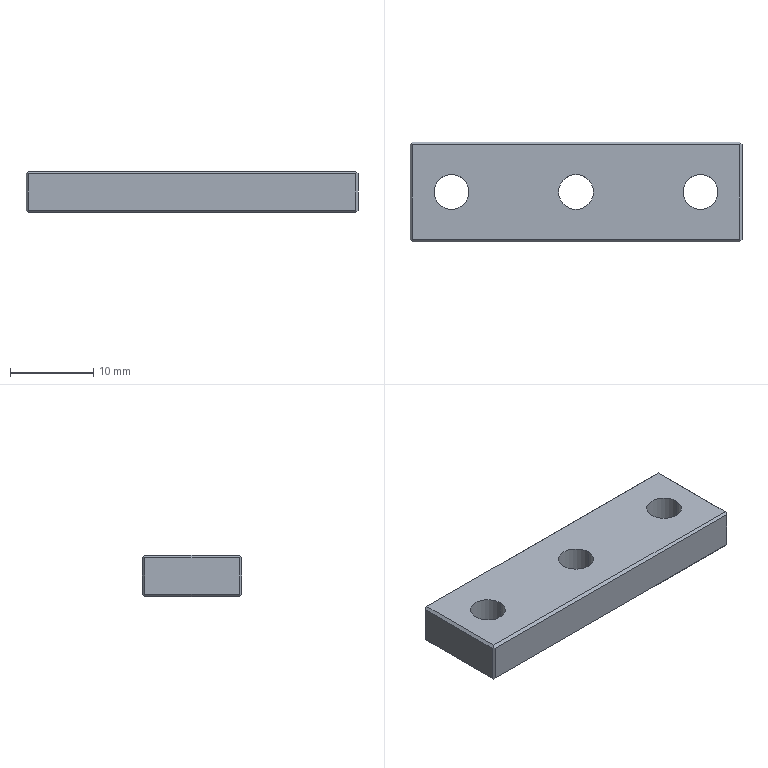Part | NX | 1 solid | 30 faces | box 40 x 12 x 5 mm | volume 2175 mm3 | plane 18 | cylinder 6 | cone 6 | commonest cylinder face diameters 4.2 x6
STEP:
#1=CARTESIAN_POINT('',(536.,16.4,-148.98));
#2=VERTEX_POINT('',#1);
#3=CARTESIAN_POINT('',(536.,16.4,-144.58));
#4=VERTEX_POINT('',#3);
#5=CARTESIAN_POINT('',(536.,16.4,-146.78));
#6=DIRECTION('',(0.,0.,1.));
#7=VECTOR('',#6,1000.);
#8=LINE('',#5,#7);
#9=EDGE_CURVE('',#2,#4,#8,.T.);
#10=ORIENTED_EDGE('',*,*,#9,.T.);
#11=CARTESIAN_POINT('',(536.,27.8,-144.58));
#12=VERTEX_POINT('',#11);
#13=CARTESIAN_POINT('',(536.,22.1,-144.58));
#14=DIRECTION('',(0.,1.,0.));
#15=VECTOR('',#14,1000.);
#16=LINE('',#13,#15);
#17=EDGE_CURVE('',#4,#12,#16,.T.);
#18=ORIENTED_EDGE('',*,*,#17,.T.);
#19=CARTESIAN_POINT('',(536.,27.8,-148.98));
#20=VERTEX_POINT('',#19);
#21=CARTESIAN_POINT('',(536.,27.8,-146.78));
#22=DIRECTION('',(0.,0.,1.));
#23=VECTOR('',#22,1000.);
#24=LINE('',#21,#23);
#25=EDGE_CURVE('',#20,#12,#24,.T.);
#26=ORIENTED_EDGE('',*,*,#25,.F.);
#27=CARTESIAN_POINT('',(536.,22.1,-148.98));
#28=DIRECTION('',(0.,1.,0.));
#29=VECTOR('',#28,1000.);
#30=LINE('',#27,#29);
#31=EDGE_CURVE('',#2,#20,#30,.T.);
#32=ORIENTED_EDGE('',*,*,#31,.F.);
#33=EDGE_LOOP('',(#10,#18,#26,#32));
#34=FACE_BOUND('',#33,.T.);
#35=CARTESIAN_POINT('',(536.,28.1,-144.28));
#36=DIRECTION('',(-1.,0.,0.));
#37=DIRECTION('',(0.,0.,1.));
#38=AXIS2_PLACEMENT_3D('',#35,#36,#37);
#39=PLANE('',#38);
#40=ADVANCED_FACE('',(#34),#39,.T.);
#41=CARTESIAN_POINT('',(575.7,28.1,-144.58));
#42=VERTEX_POINT('',#41);
#43=CARTESIAN_POINT('',(575.7,28.1,-148.98));
#44=VERTEX_POINT('',#43);
#45=CARTESIAN_POINT('',(575.7,28.1,-146.78));
#46=DIRECTION('',(0.,0.,-1.));
#47=VECTOR('',#46,1000.);
#48=LINE('',#45,#47);
#49=EDGE_CURVE('',#42,#44,#48,.T.);
#50=ORIENTED_EDGE('',*,*,#49,.T.);
#51=CARTESIAN_POINT('',(536.3,28.1,-148.98));
#52=VERTEX_POINT('',#51);
#53=CARTESIAN_POINT('',(556.,28.1,-148.98));
#54=DIRECTION('',(-1.,0.,0.));
#55=VECTOR('',#54,1000.);
#56=LINE('',#53,#55);
#57=EDGE_CURVE('',#44,#52,#56,.T.);
#58=ORIENTED_EDGE('',*,*,#57,.T.);
#59=CARTESIAN_POINT('',(536.3,28.1,-144.58));
#60=VERTEX_POINT('',#59);
#61=CARTESIAN_POINT('',(536.3,28.1,-146.78));
#62=DIRECTION('',(0.,0.,1.));
#63=VECTOR('',#62,1000.);
#64=LINE('',#61,#63);
#65=EDGE_CURVE('',#52,#60,#64,.T.);
#66=ORIENTED_EDGE('',*,*,#65,.T.);
#67=CARTESIAN_POINT('',(556.,28.1,-144.58));
#68=DIRECTION('',(-1.,0.,0.));
#69=VECTOR('',#68,1000.);
#70=LINE('',#67,#69);
#71=EDGE_CURVE('',#42,#60,#70,.T.);
#72=ORIENTED_EDGE('',*,*,#71,.F.);
#73=EDGE_LOOP('',(#50,#58,#66,#72));
#74=FACE_BOUND('',#73,.T.);
#75=CARTESIAN_POINT('',(596.,28.1,-144.28));
#76=DIRECTION('',(0.,1.,0.));
#77=DIRECTION('',(1.,0.,0.));
#78=AXIS2_PLACEMENT_3D('',#75,#76,#77);
#79=PLANE('',#78);
#80=ADVANCED_FACE('',(#74),#79,.T.);
#81=CARTESIAN_POINT('',(576.,16.4,-144.58));
#82=VERTEX_POINT('',#81);
#83=CARTESIAN_POINT('',(576.,16.4,-148.98));
#84=VERTEX_POINT('',#83);
#85=CARTESIAN_POINT('',(576.,16.4,-146.78));
#86=DIRECTION('',(0.,0.,-1.));
#87=VECTOR('',#86,1000.);
#88=LINE('',#85,#87);
#89=EDGE_CURVE('',#82,#84,#88,.T.);
#90=ORIENTED_EDGE('',*,*,#89,.T.);
#91=CARTESIAN_POINT('',(576.,27.8,-148.98));
#92=VERTEX_POINT('',#91);
#93=CARTESIAN_POINT('',(576.,22.1,-148.98));
#94=DIRECTION('',(0.,-1.,0.));
#95=VECTOR('',#94,1000.);
#96=LINE('',#93,#95);
#97=EDGE_CURVE('',#92,#84,#96,.T.);
#98=ORIENTED_EDGE('',*,*,#97,.F.);
#99=CARTESIAN_POINT('',(576.,27.8,-144.58));
#100=VERTEX_POINT('',#99);
#101=CARTESIAN_POINT('',(576.,27.8,-146.78));
#102=DIRECTION('',(0.,0.,-1.));
#103=VECTOR('',#102,1000.);
#104=LINE('',#101,#103);
#105=EDGE_CURVE('',#100,#92,#104,.T.);
#106=ORIENTED_EDGE('',*,*,#105,.F.);
#107=CARTESIAN_POINT('',(576.,22.1,-144.58));
#108=DIRECTION('',(0.,-1.,0.));
#109=VECTOR('',#108,1000.);
#110=LINE('',#107,#109);
#111=EDGE_CURVE('',#100,#82,#110,.T.);
#112=ORIENTED_EDGE('',*,*,#111,.T.);
#113=EDGE_LOOP('',(#90,#98,#106,#112));
#114=FACE_BOUND('',#113,.T.);
#115=CARTESIAN_POINT('',(576.,17.1,-144.28));
#116=DIRECTION('',(1.,0.,0.));
#117=DIRECTION('',(0.,1.,0.));
#118=AXIS2_PLACEMENT_3D('',#115,#116,#117);
#119=PLANE('',#118);
#120=ADVANCED_FACE('',(#114),#119,.T.);
#121=CARTESIAN_POINT('',(575.7,16.1,-144.58));
#122=VERTEX_POINT('',#121);
#123=CARTESIAN_POINT('',(536.3,16.1,-144.58));
#124=VERTEX_POINT('',#123);
#125=CARTESIAN_POINT('',(556.,16.1,-144.58));
#126=DIRECTION('',(-1.,0.,0.));
#127=VECTOR('',#126,1000.);
#128=LINE('',#125,#127);
#129=EDGE_CURVE('',#122,#124,#128,.T.);
#130=ORIENTED_EDGE('',*,*,#129,.T.);
#131=CARTESIAN_POINT('',(536.3,16.1,-148.98));
#132=VERTEX_POINT('',#131);
#133=CARTESIAN_POINT('',(536.3,16.1,-146.78));
#134=DIRECTION('',(0.,0.,1.));
#135=VECTOR('',#134,1000.);
#136=LINE('',#133,#135);
#137=EDGE_CURVE('',#132,#124,#136,.T.);
#138=ORIENTED_EDGE('',*,*,#137,.F.);
#139=CARTESIAN_POINT('',(575.7,16.1,-148.98));
#140=VERTEX_POINT('',#139);
#141=CARTESIAN_POINT('',(556.,16.1,-148.98));
#142=DIRECTION('',(-1.,0.,0.));
#143=VECTOR('',#142,1000.);
#144=LINE('',#141,#143);
#145=EDGE_CURVE('',#140,#132,#144,.T.);
#146=ORIENTED_EDGE('',*,*,#145,.F.);
#147=CARTESIAN_POINT('',(575.7,16.1,-146.78));
#148=DIRECTION('',(0.,0.,-1.));
#149=VECTOR('',#148,1000.);
#150=LINE('',#147,#149);
#151=EDGE_CURVE('',#122,#140,#150,.T.);
#152=ORIENTED_EDGE('',*,*,#151,.F.);
#153=EDGE_LOOP('',(#130,#138,#146,#152));
#154=FACE_BOUND('',#153,.T.);
#155=CARTESIAN_POINT('',(516.,16.1,-144.28));
#156=DIRECTION('',(0.,-1.,0.));
#157=DIRECTION('',(0.,0.,-1.));
#158=AXIS2_PLACEMENT_3D('',#155,#156,#157);
#159=PLANE('',#158);
#160=ADVANCED_FACE('',(#154),#159,.T.);
#161=ORIENTED_EDGE('',*,*,#89,.F.);
#162=CARTESIAN_POINT('',(575.85,16.25,-144.43));
#163=VERTEX_POINT('',#162);
#164=CARTESIAN_POINT('',(555.747,-3.853,-124.327));
#165=DIRECTION('',(-0.5774,-0.5774,0.5774));
#166=VECTOR('',#165,1000.);
#167=LINE('',#164,#166);
#168=EDGE_CURVE('',#82,#163,#167,.T.);
#169=ORIENTED_EDGE('',*,*,#168,.T.);
#170=CARTESIAN_POINT('',(555.747,-3.853,-164.533));
#171=DIRECTION('',(-0.5774,-0.5774,-0.5774));
#172=VECTOR('',#171,1000.);
#173=LINE('',#170,#172);
#174=EDGE_CURVE('',#163,#122,#173,.T.);
#175=ORIENTED_EDGE('',*,*,#174,.T.);
#176=ORIENTED_EDGE('',*,*,#151,.T.);
#177=CARTESIAN_POINT('',(575.85,16.25,-149.13));
#178=VERTEX_POINT('',#177);
#179=CARTESIAN_POINT('',(555.747,-3.853,-129.027));
#180=DIRECTION('',(-0.5774,-0.5774,0.5774));
#181=VECTOR('',#180,1000.);
#182=LINE('',#179,#181);
#183=EDGE_CURVE('',#178,#140,#182,.T.);
#184=ORIENTED_EDGE('',*,*,#183,.F.);
#185=CARTESIAN_POINT('',(555.747,-3.853,-169.233));
#186=DIRECTION('',(-0.5774,-0.5774,-0.5774));
#187=VECTOR('',#186,1000.);
#188=LINE('',#185,#187);
#189=EDGE_CURVE('',#84,#178,#188,.T.);
#190=ORIENTED_EDGE('',*,*,#189,.F.);
#191=EDGE_LOOP('',(#161,#169,#175,#176,#184,#190));
#192=FACE_BOUND('',#191,.T.);
#193=CARTESIAN_POINT('',(575.85,16.25,-146.78));
#194=DIRECTION('',(0.7071,-0.7071,0.));
#195=DIRECTION('',(0.,0.,-1.));
#196=AXIS2_PLACEMENT_3D('',#193,#194,#195);
#197=PLANE('',#196);
#198=ADVANCED_FACE('',(#192),#197,.T.);
#199=ORIENTED_EDGE('',*,*,#49,.F.);
#200=CARTESIAN_POINT('',(575.85,27.95,-144.43));
#201=VERTEX_POINT('',#200);
#202=CARTESIAN_POINT('',(607.653,-3.853,-112.627));
#203=DIRECTION('',(-0.5774,0.5774,-0.5774));
#204=VECTOR('',#203,1000.);
#205=LINE('',#202,#204);
#206=EDGE_CURVE('',#201,#42,#205,.T.);
#207=ORIENTED_EDGE('',*,*,#206,.F.);
#208=CARTESIAN_POINT('',(607.653,-3.853,-176.233));
#209=DIRECTION('',(0.5774,-0.5774,-0.5774));
#210=VECTOR('',#209,1000.);
#211=LINE('',#208,#210);
#212=EDGE_CURVE('',#201,#100,#211,.T.);
#213=ORIENTED_EDGE('',*,*,#212,.T.);
#214=ORIENTED_EDGE('',*,*,#105,.T.);
#215=CARTESIAN_POINT('',(575.85,27.95,-149.13));
#216=VERTEX_POINT('',#215);
#217=CARTESIAN_POINT('',(607.653,-3.853,-117.327));
#218=DIRECTION('',(0.5774,-0.5774,0.5774));
#219=VECTOR('',#218,1000.);
#220=LINE('',#217,#219);
#221=EDGE_CURVE('',#216,#92,#220,.T.);
#222=ORIENTED_EDGE('',*,*,#221,.F.);
#223=CARTESIAN_POINT('',(607.653,-3.853,-180.933));
#224=DIRECTION('',(-0.5774,0.5774,0.5774));
#225=VECTOR('',#224,1000.);
#226=LINE('',#223,#225);
#227=EDGE_CURVE('',#216,#44,#226,.T.);
#228=ORIENTED_EDGE('',*,*,#227,.T.);
#229=EDGE_LOOP('',(#199,#207,#213,#214,#222,#228));
#230=FACE_BOUND('',#229,.T.);
#231=CARTESIAN_POINT('',(575.85,27.95,-146.78));
#232=DIRECTION('',(0.7071,0.7071,0.));
#233=DIRECTION('',(0.,0.,-1.));
#234=AXIS2_PLACEMENT_3D('',#231,#232,#233);
#235=PLANE('',#234);
#236=ADVANCED_FACE('',(#230),#235,.T.);
#237=ORIENTED_EDGE('',*,*,#25,.T.);
#238=CARTESIAN_POINT('',(536.15,27.95,-144.43));
#239=VERTEX_POINT('',#238);
#240=CARTESIAN_POINT('',(504.347,-3.853,-176.233));
#241=DIRECTION('',(-0.5774,-0.5774,-0.5774));
#242=VECTOR('',#241,1000.);
#243=LINE('',#240,#242);
#244=EDGE_CURVE('',#239,#12,#243,.T.);
#245=ORIENTED_EDGE('',*,*,#244,.F.);
#246=CARTESIAN_POINT('',(504.347,-3.853,-112.627));
#247=DIRECTION('',(0.5774,0.5774,-0.5774));
#248=VECTOR('',#247,1000.);
#249=LINE('',#246,#248);
#250=EDGE_CURVE('',#239,#60,#249,.T.);
#251=ORIENTED_EDGE('',*,*,#250,.T.);
#252=ORIENTED_EDGE('',*,*,#65,.F.);
#253=CARTESIAN_POINT('',(536.15,27.95,-149.13));
#254=VERTEX_POINT('',#253);
#255=CARTESIAN_POINT('',(504.347,-3.853,-180.933));
#256=DIRECTION('',(0.5774,0.5774,0.5774));
#257=VECTOR('',#256,1000.);
#258=LINE('',#255,#257);
#259=EDGE_CURVE('',#254,#52,#258,.T.);
#260=ORIENTED_EDGE('',*,*,#259,.F.);
#261=CARTESIAN_POINT('',(504.347,-3.853,-117.327));
#262=DIRECTION('',(-0.5774,-0.5774,0.5774));
#263=VECTOR('',#262,1000.);
#264=LINE('',#261,#263);
#265=EDGE_CURVE('',#254,#20,#264,.T.);
#266=ORIENTED_EDGE('',*,*,#265,.T.);
#267=EDGE_LOOP('',(#237,#245,#251,#252,#260,#266));
#268=FACE_BOUND('',#267,.T.);
#269=CARTESIAN_POINT('',(536.15,27.95,-146.78));
#270=DIRECTION('',(0.7071,-0.7071,0.));
#271=DIRECTION('',(0.,0.,-1.));
#272=AXIS2_PLACEMENT_3D('',#269,#270,#271);
#273=PLANE('',#272);
#274=ADVANCED_FACE('',(#268),#273,.F.);
#275=ORIENTED_EDGE('',*,*,#9,.F.);
#276=CARTESIAN_POINT('',(536.15,16.25,-149.13));
#277=VERTEX_POINT('',#276);
#278=CARTESIAN_POINT('',(556.253,-3.853,-169.233));
#279=DIRECTION('',(-0.5774,0.5774,0.5774));
#280=VECTOR('',#279,1000.);
#281=LINE('',#278,#280);
#282=EDGE_CURVE('',#277,#2,#281,.T.);
#283=ORIENTED_EDGE('',*,*,#282,.F.);
#284=CARTESIAN_POINT('',(556.253,-3.853,-129.027));
#285=DIRECTION('',(-0.5774,0.5774,-0.5774));
#286=VECTOR('',#285,1000.);
#287=LINE('',#284,#286);
#288=EDGE_CURVE('',#132,#277,#287,.T.);
#289=ORIENTED_EDGE('',*,*,#288,.F.);
#290=ORIENTED_EDGE('',*,*,#137,.T.);
#291=CARTESIAN_POINT('',(536.15,16.25,-144.43));
#292=VERTEX_POINT('',#291);
#293=CARTESIAN_POINT('',(556.253,-3.853,-164.533));
#294=DIRECTION('',(-0.5774,0.5774,0.5774));
#295=VECTOR('',#294,1000.);
#296=LINE('',#293,#295);
#297=EDGE_CURVE('',#124,#292,#296,.T.);
#298=ORIENTED_EDGE('',*,*,#297,.T.);
#299=CARTESIAN_POINT('',(538.281,14.119,-142.299));
#300=DIRECTION('',(-0.5774,0.5774,-0.5774));
#301=VECTOR('',#300,1000.);
#302=LINE('',#299,#301);
#303=EDGE_CURVE('',#292,#4,#302,.T.);
#304=ORIENTED_EDGE('',*,*,#303,.T.);
#305=EDGE_LOOP('',(#275,#283,#289,#290,#298,#304));
#306=FACE_BOUND('',#305,.T.);
#307=CARTESIAN_POINT('',(536.15,16.25,-146.78));
#308=DIRECTION('',(-0.7071,-0.7071,0.));
#309=DIRECTION('',(-0.7071,0.7071,0.));
#310=AXIS2_PLACEMENT_3D('',#307,#308,#309);
#311=PLANE('',#310);
#312=ADVANCED_FACE('',(#306),#311,.T.);
#313=CARTESIAN_POINT('',(575.7,27.8,-149.28));
#314=VERTEX_POINT('',#313);
#315=CARTESIAN_POINT('',(575.7,16.4,-149.28));
#316=VERTEX_POINT('',#315);
#317=CARTESIAN_POINT('',(575.7,22.1,-149.28));
#318=DIRECTION('',(0.,-1.,0.));
#319=VECTOR('',#318,1000.);
#320=LINE('',#317,#319);
#321=EDGE_CURVE('',#314,#316,#320,.T.);
#322=ORIENTED_EDGE('',*,*,#321,.T.);
#323=CARTESIAN_POINT('',(536.3,16.4,-149.28));
#324=VERTEX_POINT('',#323);
#325=CARTESIAN_POINT('',(556.,16.4,-149.28));
#326=DIRECTION('',(-1.,0.,0.));
#327=VECTOR('',#326,1000.);
#328=LINE('',#325,#327);
#329=EDGE_CURVE('',#316,#324,#328,.T.);
#330=ORIENTED_EDGE('',*,*,#329,.T.);
#331=CARTESIAN_POINT('',(536.3,27.8,-149.28));
#332=VERTEX_POINT('',#331);
#333=CARTESIAN_POINT('',(536.3,22.1,-149.28));
#334=DIRECTION('',(0.,1.,0.));
#335=VECTOR('',#334,1000.);
#336=LINE('',#333,#335);
#337=EDGE_CURVE('',#324,#332,#336,.T.);
#338=ORIENTED_EDGE('',*,*,#337,.T.);
#339=CARTESIAN_POINT('',(556.,27.8,-149.28));
#340=DIRECTION('',(-1.,0.,0.));
#341=VECTOR('',#340,1000.);
#342=LINE('',#339,#341);
#343=EDGE_CURVE('',#314,#332,#342,.T.);
#344=ORIENTED_EDGE('',*,*,#343,.F.);
#345=EDGE_LOOP('',(#322,#330,#338,#344));
#346=FACE_BOUND('',#345,.T.);
#347=CARTESIAN_POINT('',(558.86,22.1,-149.28));
#348=VERTEX_POINT('',#347);
#349=CARTESIAN_POINT('',(553.14,22.1,-149.28));
#350=VERTEX_POINT('',#349);
#351=CARTESIAN_POINT('',(556.,22.1,-149.28));
#352=DIRECTION('',(0.,0.,-1.));
#353=DIRECTION('',(-1.,0.,0.));
#354=AXIS2_PLACEMENT_3D('',#351,#352,#353);
#355=CIRCLE('',#354,2.86);
#356=EDGE_CURVE('',#348,#350,#355,.T.);
#357=ORIENTED_EDGE('',*,*,#356,.F.);
#358=CARTESIAN_POINT('',(556.,22.1,-149.28));
#359=DIRECTION('',(0.,0.,-1.));
#360=DIRECTION('',(-1.,0.,0.));
#361=AXIS2_PLACEMENT_3D('',#358,#359,#360);
#362=CIRCLE('',#361,2.86);
#363=EDGE_CURVE('',#350,#348,#362,.T.);
#364=ORIENTED_EDGE('',*,*,#363,.F.);
#365=EDGE_LOOP('',(#357,#364));
#366=FACE_BOUND('',#365,.T.);
#367=CARTESIAN_POINT('',(573.86,22.1,-149.28));
#368=VERTEX_POINT('',#367);
#369=CARTESIAN_POINT('',(568.14,22.1,-149.28));
#370=VERTEX_POINT('',#369);
#371=CARTESIAN_POINT('',(571.,22.1,-149.28));
#372=DIRECTION('',(0.,0.,-1.));
#373=DIRECTION('',(-1.,0.,0.));
#374=AXIS2_PLACEMENT_3D('',#371,#372,#373);
#375=CIRCLE('',#374,2.86);
#376=EDGE_CURVE('',#368,#370,#375,.T.);
#377=ORIENTED_EDGE('',*,*,#376,.F.);
#378=CARTESIAN_POINT('',(571.,22.1,-149.28));
#379=DIRECTION('',(0.,0.,-1.));
#380=DIRECTION('',(-1.,0.,0.));
#381=AXIS2_PLACEMENT_3D('',#378,#379,#380);
#382=CIRCLE('',#381,2.86);
#383=EDGE_CURVE('',#370,#368,#382,.T.);
#384=ORIENTED_EDGE('',*,*,#383,.F.);
#385=EDGE_LOOP('',(#377,#384));
#386=FACE_BOUND('',#385,.T.);
#387=CARTESIAN_POINT('',(543.86,22.1,-149.28));
#388=VERTEX_POINT('',#387);
#389=CARTESIAN_POINT('',(538.14,22.1,-149.28));
#390=VERTEX_POINT('',#389);
#391=CARTESIAN_POINT('',(541.,22.1,-149.28));
#392=DIRECTION('',(0.,0.,-1.));
#393=DIRECTION('',(-1.,0.,0.));
#394=AXIS2_PLACEMENT_3D('',#391,#392,#393);
#395=CIRCLE('',#394,2.86);
#396=EDGE_CURVE('',#388,#390,#395,.T.);
#397=ORIENTED_EDGE('',*,*,#396,.F.);
#398=CARTESIAN_POINT('',(541.,22.1,-149.28));
#399=DIRECTION('',(0.,0.,-1.));
#400=DIRECTION('',(-1.,0.,0.));
#401=AXIS2_PLACEMENT_3D('',#398,#399,#400);
#402=CIRCLE('',#401,2.86);
#403=EDGE_CURVE('',#390,#388,#402,.T.);
#404=ORIENTED_EDGE('',*,*,#403,.F.);
#405=EDGE_LOOP('',(#397,#404));
#406=FACE_BOUND('',#405,.T.);
#407=CARTESIAN_POINT('',(538.281,-3.853,-149.28));
#408=DIRECTION('',(0.,0.,-1.));
#409=DIRECTION('',(0.,-1.,0.));
#410=AXIS2_PLACEMENT_3D('',#407,#408,#409);
#411=PLANE('',#410);
#412=ADVANCED_FACE('',(#346,#366,#386,#406),#411,.T.);
#413=CARTESIAN_POINT('',(573.1,22.1,-148.841));
#414=VERTEX_POINT('',#413);
#415=CARTESIAN_POINT('',(568.9,22.1,-148.841));
#416=VERTEX_POINT('',#415);
#417=CARTESIAN_POINT('',(571.,22.1,-148.841));
#418=DIRECTION('',(0.,0.,-1.));
#419=DIRECTION('',(-1.,0.,0.));
#420=AXIS2_PLACEMENT_3D('',#417,#418,#419);
#421=CIRCLE('',#420,2.1);
#422=EDGE_CURVE('',#414,#416,#421,.T.);
#423=ORIENTED_EDGE('',*,*,#422,.T.);
#424=CARTESIAN_POINT('',(568.9,22.1,-144.28));
#425=VERTEX_POINT('',#424);
#426=CARTESIAN_POINT('',(568.9,22.1,-149.28));
#427=DIRECTION('',(0.,0.,-1.));
#428=VECTOR('',#427,1000.);
#429=LINE('',#426,#428);
#430=EDGE_CURVE('',#416,#425,#429,.F.);
#431=ORIENTED_EDGE('',*,*,#430,.T.);
#432=CARTESIAN_POINT('',(573.1,22.1,-144.28));
#433=VERTEX_POINT('',#432);
#434=CARTESIAN_POINT('',(571.,22.1,-144.28));
#435=DIRECTION('',(0.,0.,-1.));
#436=DIRECTION('',(-1.,0.,0.));
#437=AXIS2_PLACEMENT_3D('',#434,#435,#436);
#438=CIRCLE('',#437,2.1);
#439=EDGE_CURVE('',#433,#425,#438,.T.);
#440=ORIENTED_EDGE('',*,*,#439,.F.);
#441=CARTESIAN_POINT('',(573.1,22.1,-149.28));
#442=DIRECTION('',(0.,0.,-1.));
#443=VECTOR('',#442,1000.);
#444=LINE('',#441,#443);
#445=EDGE_CURVE('',#414,#433,#444,.F.);
#446=ORIENTED_EDGE('',*,*,#445,.F.);
#447=EDGE_LOOP('',(#423,#431,#440,#446));
#448=FACE_BOUND('',#447,.T.);
#449=CARTESIAN_POINT('',(571.,22.1,-149.28));
#450=DIRECTION('',(0.,0.,-1.));
#451=DIRECTION('',(-1.,0.,0.));
#452=AXIS2_PLACEMENT_3D('',#449,#450,#451);
#453=CYLINDRICAL_SURFACE('',#452,2.1);
#454=ADVANCED_FACE('',(#448),#453,.F.);
#455=ORIENTED_EDGE('',*,*,#422,.F.);
#456=CARTESIAN_POINT('',(573.1,22.1,-148.841));
#457=DIRECTION('',(0.866,0.,-0.5));
#458=VECTOR('',#457,1000.);
#459=LINE('',#456,#458);
#460=EDGE_CURVE('',#368,#414,#459,.F.);
#461=ORIENTED_EDGE('',*,*,#460,.F.);
#462=ORIENTED_EDGE('',*,*,#376,.T.);
#463=CARTESIAN_POINT('',(568.9,22.1,-148.841));
#464=DIRECTION('',(-0.866,0.,-0.5));
#465=VECTOR('',#464,1000.);
#466=LINE('',#463,#465);
#467=EDGE_CURVE('',#370,#416,#466,.F.);
#468=ORIENTED_EDGE('',*,*,#467,.T.);
#469=EDGE_LOOP('',(#455,#461,#462,#468));
#470=FACE_BOUND('',#469,.T.);
#471=CARTESIAN_POINT('',(571.,22.1,-148.841));
#472=DIRECTION('',(0.,0.,-1.));
#473=DIRECTION('',(-1.,0.,0.));
#474=AXIS2_PLACEMENT_3D('',#471,#472,#473);
#475=CONICAL_SURFACE('',#474,2.1,1.047);
#476=ADVANCED_FACE('',(#470),#475,.F.);
#477=CARTESIAN_POINT('',(558.1,22.1,-148.841));
#478=VERTEX_POINT('',#477);
#479=CARTESIAN_POINT('',(553.9,22.1,-148.841));
#480=VERTEX_POINT('',#479);
#481=CARTESIAN_POINT('',(556.,22.1,-148.841));
#482=DIRECTION('',(0.,0.,-1.));
#483=DIRECTION('',(-1.,0.,0.));
#484=AXIS2_PLACEMENT_3D('',#481,#482,#483);
#485=CIRCLE('',#484,2.1);
#486=EDGE_CURVE('',#478,#480,#485,.T.);
#487=ORIENTED_EDGE('',*,*,#486,.T.);
#488=CARTESIAN_POINT('',(553.9,22.1,-144.28));
#489=VERTEX_POINT('',#488);
#490=CARTESIAN_POINT('',(553.9,22.1,-149.28));
#491=DIRECTION('',(0.,0.,-1.));
#492=VECTOR('',#491,1000.);
#493=LINE('',#490,#492);
#494=EDGE_CURVE('',#480,#489,#493,.F.);
#495=ORIENTED_EDGE('',*,*,#494,.T.);
#496=CARTESIAN_POINT('',(558.1,22.1,-144.28));
#497=VERTEX_POINT('',#496);
#498=CARTESIAN_POINT('',(556.,22.1,-144.28));
#499=DIRECTION('',(0.,0.,-1.));
#500=DIRECTION('',(-1.,0.,0.));
#501=AXIS2_PLACEMENT_3D('',#498,#499,#500);
#502=CIRCLE('',#501,2.1);
#503=EDGE_CURVE('',#497,#489,#502,.T.);
#504=ORIENTED_EDGE('',*,*,#503,.F.);
#505=CARTESIAN_POINT('',(558.1,22.1,-149.28));
#506=DIRECTION('',(0.,0.,-1.));
#507=VECTOR('',#506,1000.);
#508=LINE('',#505,#507);
#509=EDGE_CURVE('',#478,#497,#508,.F.);
#510=ORIENTED_EDGE('',*,*,#509,.F.);
#511=EDGE_LOOP('',(#487,#495,#504,#510));
#512=FACE_BOUND('',#511,.T.);
#513=CARTESIAN_POINT('',(556.,22.1,-149.28));
#514=DIRECTION('',(0.,0.,-1.));
#515=DIRECTION('',(-1.,0.,0.));
#516=AXIS2_PLACEMENT_3D('',#513,#514,#515);
#517=CYLINDRICAL_SURFACE('',#516,2.1);
#518=ADVANCED_FACE('',(#512),#517,.F.);
#519=ORIENTED_EDGE('',*,*,#486,.F.);
#520=CARTESIAN_POINT('',(558.1,22.1,-148.841));
#521=DIRECTION('',(0.866,0.,-0.5));
#522=VECTOR('',#521,1000.);
#523=LINE('',#520,#522);
#524=EDGE_CURVE('',#348,#478,#523,.F.);
#525=ORIENTED_EDGE('',*,*,#524,.F.);
#526=ORIENTED_EDGE('',*,*,#356,.T.);
#527=CARTESIAN_POINT('',(553.9,22.1,-148.841));
#528=DIRECTION('',(-0.866,0.,-0.5));
#529=VECTOR('',#528,1000.);
#530=LINE('',#527,#529);
#531=EDGE_CURVE('',#350,#480,#530,.F.);
#532=ORIENTED_EDGE('',*,*,#531,.T.);
#533=EDGE_LOOP('',(#519,#525,#526,#532));
#534=FACE_BOUND('',#533,.T.);
#535=CARTESIAN_POINT('',(556.,22.1,-148.841));
#536=DIRECTION('',(0.,0.,-1.));
#537=DIRECTION('',(-1.,0.,0.));
#538=AXIS2_PLACEMENT_3D('',#535,#536,#537);
#539=CONICAL_SURFACE('',#538,2.1,1.047);
#540=ADVANCED_FACE('',(#534),#539,.F.);
#541=CARTESIAN_POINT('',(543.1,22.1,-148.841));
#542=VERTEX_POINT('',#541);
#543=CARTESIAN_POINT('',(538.9,22.1,-148.841));
#544=VERTEX_POINT('',#543);
#545=CARTESIAN_POINT('',(541.,22.1,-148.841));
#546=DIRECTION('',(0.,0.,-1.));
#547=DIRECTION('',(-1.,0.,0.));
#548=AXIS2_PLACEMENT_3D('',#545,#546,#547);
#549=CIRCLE('',#548,2.1);
#550=EDGE_CURVE('',#542,#544,#549,.T.);
#551=ORIENTED_EDGE('',*,*,#550,.T.);
#552=CARTESIAN_POINT('',(538.9,22.1,-144.28));
#553=VERTEX_POINT('',#552);
#554=CARTESIAN_POINT('',(538.9,22.1,-149.28));
#555=DIRECTION('',(0.,0.,-1.));
#556=VECTOR('',#555,1000.);
#557=LINE('',#554,#556);
#558=EDGE_CURVE('',#544,#553,#557,.F.);
#559=ORIENTED_EDGE('',*,*,#558,.T.);
#560=CARTESIAN_POINT('',(543.1,22.1,-144.28));
#561=VERTEX_POINT('',#560);
#562=CARTESIAN_POINT('',(541.,22.1,-144.28));
#563=DIRECTION('',(0.,0.,-1.));
#564=DIRECTION('',(-1.,0.,0.));
#565=AXIS2_PLACEMENT_3D('',#562,#563,#564);
#566=CIRCLE('',#565,2.1);
#567=EDGE_CURVE('',#561,#553,#566,.T.);
#568=ORIENTED_EDGE('',*,*,#567,.F.);
#569=CARTESIAN_POINT('',(543.1,22.1,-149.28));
#570=DIRECTION('',(0.,0.,-1.));
#571=VECTOR('',#570,1000.);
#572=LINE('',#569,#571);
#573=EDGE_CURVE('',#542,#561,#572,.F.);
#574=ORIENTED_EDGE('',*,*,#573,.F.);
#575=EDGE_LOOP('',(#551,#559,#568,#574));
#576=FACE_BOUND('',#575,.T.);
#577=CARTESIAN_POINT('',(541.,22.1,-149.28));
#578=DIRECTION('',(0.,0.,-1.));
#579=DIRECTION('',(-1.,0.,0.));
#580=AXIS2_PLACEMENT_3D('',#577,#578,#579);
#581=CYLINDRICAL_SURFACE('',#580,2.1);
#582=ADVANCED_FACE('',(#576),#581,.F.);
#583=ORIENTED_EDGE('',*,*,#550,.F.);
#584=CARTESIAN_POINT('',(543.1,22.1,-148.841));
#585=DIRECTION('',(0.866,0.,-0.5));
#586=VECTOR('',#585,1000.);
#587=LINE('',#584,#586);
#588=EDGE_CURVE('',#388,#542,#587,.F.);
#589=ORIENTED_EDGE('',*,*,#588,.F.);
#590=ORIENTED_EDGE('',*,*,#396,.T.);
#591=CARTESIAN_POINT('',(538.9,22.1,-148.841));
#592=DIRECTION('',(-0.866,0.,-0.5));
#593=VECTOR('',#592,1000.);
#594=LINE('',#591,#593);
#595=EDGE_CURVE('',#390,#544,#594,.F.);
#596=ORIENTED_EDGE('',*,*,#595,.T.);
#597=EDGE_LOOP('',(#583,#589,#590,#596));
#598=FACE_BOUND('',#597,.T.);
#599=CARTESIAN_POINT('',(541.,22.1,-148.841));
#600=DIRECTION('',(0.,0.,-1.));
#601=DIRECTION('',(-1.,0.,0.));
#602=AXIS2_PLACEMENT_3D('',#599,#600,#601);
#603=CONICAL_SURFACE('',#602,2.1,1.047);
#604=ADVANCED_FACE('',(#598),#603,.F.);
#605=ORIENTED_EDGE('',*,*,#343,.T.);
#606=CARTESIAN_POINT('',(567.953,-3.853,-180.933));
#607=DIRECTION('',(0.5774,-0.5774,-0.5774));
#608=VECTOR('',#607,1000.);
#609=LINE('',#606,#608);
#610=EDGE_CURVE('',#254,#332,#609,.T.);
#611=ORIENTED_EDGE('',*,*,#610,.F.);
#612=ORIENTED_EDGE('',*,*,#259,.T.);
#613=ORIENTED_EDGE('',*,*,#57,.F.);
#614=ORIENTED_EDGE('',*,*,#227,.F.);
#615=CARTESIAN_POINT('',(544.047,-3.853,-180.933));
#616=DIRECTION('',(-0.5774,-0.5774,-0.5774));
#617=VECTOR('',#616,1000.);
#618=LINE('',#615,#617);
#619=EDGE_CURVE('',#216,#314,#618,.T.);
#620=ORIENTED_EDGE('',*,*,#619,.T.);
#621=EDGE_LOOP('',(#605,#611,#612,#613,#614,#620));
#622=FACE_BOUND('',#621,.T.);
#623=CARTESIAN_POINT('',(556.,27.95,-149.13));
#624=DIRECTION('',(0.,-0.7071,0.7071));
#625=DIRECTION('',(-1.,0.,0.));
#626=AXIS2_PLACEMENT_3D('',#623,#624,#625);
#627=PLANE('',#626);
#628=ADVANCED_FACE('',(#622),#627,.F.);
#629=ORIENTED_EDGE('',*,*,#337,.F.);
#630=CARTESIAN_POINT('',(516.047,-3.853,-129.027));
#631=DIRECTION('',(-0.5774,-0.5774,0.5774));
#632=VECTOR('',#631,1000.);
#633=LINE('',#630,#632);
#634=EDGE_CURVE('',#324,#277,#633,.T.);
#635=ORIENTED_EDGE('',*,*,#634,.T.);
#636=ORIENTED_EDGE('',*,*,#282,.T.);
#637=ORIENTED_EDGE('',*,*,#31,.T.);
#638=ORIENTED_EDGE('',*,*,#265,.F.);
#639=ORIENTED_EDGE('',*,*,#610,.T.);
#640=EDGE_LOOP('',(#629,#635,#636,#637,#638,#639));
#641=FACE_BOUND('',#640,.T.);
#642=CARTESIAN_POINT('',(536.15,22.1,-149.13));
#643=DIRECTION('',(-0.7071,0.,-0.7071));
#644=DIRECTION('',(-0.7071,0.,0.7071));
#645=AXIS2_PLACEMENT_3D('',#642,#643,#644);
#646=PLANE('',#645);
#647=ADVANCED_FACE('',(#641),#646,.T.);
#648=ORIENTED_EDGE('',*,*,#329,.F.);
#649=CARTESIAN_POINT('',(595.953,-3.853,-129.027));
#650=DIRECTION('',(-0.5774,0.5774,-0.5774));
#651=VECTOR('',#650,1000.);
#652=LINE('',#649,#651);
#653=EDGE_CURVE('',#178,#316,#652,.T.);
#654=ORIENTED_EDGE('',*,*,#653,.F.);
#655=ORIENTED_EDGE('',*,*,#183,.T.);
#656=ORIENTED_EDGE('',*,*,#145,.T.);
#657=ORIENTED_EDGE('',*,*,#288,.T.);
#658=ORIENTED_EDGE('',*,*,#634,.F.);
#659=EDGE_LOOP('',(#648,#654,#655,#656,#657,#658));
#660=FACE_BOUND('',#659,.T.);
#661=CARTESIAN_POINT('',(556.,16.25,-149.13));
#662=DIRECTION('',(0.,-0.7071,-0.7071));
#663=DIRECTION('',(0.,-0.7071,0.7071));
#664=AXIS2_PLACEMENT_3D('',#661,#662,#663);
#665=PLANE('',#664);
#666=ADVANCED_FACE('',(#660),#665,.T.);
#667=ORIENTED_EDGE('',*,*,#321,.F.);
#668=ORIENTED_EDGE('',*,*,#619,.F.);
#669=ORIENTED_EDGE('',*,*,#221,.T.);
#670=ORIENTED_EDGE('',*,*,#97,.T.);
#671=ORIENTED_EDGE('',*,*,#189,.T.);
#672=ORIENTED_EDGE('',*,*,#653,.T.);
#673=EDGE_LOOP('',(#667,#668,#669,#670,#671,#672));
#674=FACE_BOUND('',#673,.T.);
#675=CARTESIAN_POINT('',(575.85,22.1,-149.13));
#676=DIRECTION('',(0.7071,0.,-0.7071));
#677=DIRECTION('',(0.,-1.,0.));
#678=AXIS2_PLACEMENT_3D('',#675,#676,#677);
#679=PLANE('',#678);
#680=ADVANCED_FACE('',(#674),#679,.T.);
#681=ORIENTED_EDGE('',*,*,#494,.F.);
#682=CARTESIAN_POINT('',(556.,22.1,-148.841));
#683=DIRECTION('',(0.,0.,-1.));
#684=DIRECTION('',(-1.,0.,0.));
#685=AXIS2_PLACEMENT_3D('',#682,#683,#684);
#686=CIRCLE('',#685,2.1);
#687=EDGE_CURVE('',#480,#478,#686,.T.);
#688=ORIENTED_EDGE('',*,*,#687,.T.);
#689=ORIENTED_EDGE('',*,*,#509,.T.);
#690=CARTESIAN_POINT('',(556.,22.1,-144.28));
#691=DIRECTION('',(0.,0.,-1.));
#692=DIRECTION('',(-1.,0.,0.));
#693=AXIS2_PLACEMENT_3D('',#690,#691,#692);
#694=CIRCLE('',#693,2.1);
#695=EDGE_CURVE('',#489,#497,#694,.T.);
#696=ORIENTED_EDGE('',*,*,#695,.F.);
#697=EDGE_LOOP('',(#681,#688,#689,#696));
#698=FACE_BOUND('',#697,.T.);
#699=CARTESIAN_POINT('',(556.,22.1,-149.28));
#700=DIRECTION('',(0.,0.,-1.));
#701=DIRECTION('',(-1.,0.,0.));
#702=AXIS2_PLACEMENT_3D('',#699,#700,#701);
#703=CYLINDRICAL_SURFACE('',#702,2.1);
#704=ADVANCED_FACE('',(#698),#703,.F.);
#705=ORIENTED_EDGE('',*,*,#467,.F.);
#706=ORIENTED_EDGE('',*,*,#383,.T.);
#707=ORIENTED_EDGE('',*,*,#460,.T.);
#708=CARTESIAN_POINT('',(571.,22.1,-148.841));
#709=DIRECTION('',(0.,0.,-1.));
#710=DIRECTION('',(-1.,0.,0.));
#711=AXIS2_PLACEMENT_3D('',#708,#709,#710);
#712=CIRCLE('',#711,2.1);
#713=EDGE_CURVE('',#416,#414,#712,.T.);
#714=ORIENTED_EDGE('',*,*,#713,.F.);
#715=EDGE_LOOP('',(#705,#706,#707,#714));
#716=FACE_BOUND('',#715,.T.);
#717=CARTESIAN_POINT('',(571.,22.1,-148.841));
#718=DIRECTION('',(0.,0.,-1.));
#719=DIRECTION('',(-1.,0.,0.));
#720=AXIS2_PLACEMENT_3D('',#717,#718,#719);
#721=CONICAL_SURFACE('',#720,2.1,1.047);
#722=ADVANCED_FACE('',(#716),#721,.F.);
#723=ORIENTED_EDGE('',*,*,#531,.F.);
#724=ORIENTED_EDGE('',*,*,#363,.T.);
#725=ORIENTED_EDGE('',*,*,#524,.T.);
#726=ORIENTED_EDGE('',*,*,#687,.F.);
#727=EDGE_LOOP('',(#723,#724,#725,#726));
#728=FACE_BOUND('',#727,.T.);
#729=CARTESIAN_POINT('',(556.,22.1,-148.841));
#730=DIRECTION('',(0.,0.,-1.));
#731=DIRECTION('',(-1.,0.,0.));
#732=AXIS2_PLACEMENT_3D('',#729,#730,#731);
#733=CONICAL_SURFACE('',#732,2.1,1.047);
#734=ADVANCED_FACE('',(#728),#733,.F.);
#735=ORIENTED_EDGE('',*,*,#595,.F.);
#736=ORIENTED_EDGE('',*,*,#403,.T.);
#737=ORIENTED_EDGE('',*,*,#588,.T.);
#738=CARTESIAN_POINT('',(541.,22.1,-148.841));
#739=DIRECTION('',(0.,0.,-1.));
#740=DIRECTION('',(-1.,0.,0.));
#741=AXIS2_PLACEMENT_3D('',#738,#739,#740);
#742=CIRCLE('',#741,2.1);
#743=EDGE_CURVE('',#544,#542,#742,.T.);
#744=ORIENTED_EDGE('',*,*,#743,.F.);
#745=EDGE_LOOP('',(#735,#736,#737,#744));
#746=FACE_BOUND('',#745,.T.);
#747=CARTESIAN_POINT('',(541.,22.1,-148.841));
#748=DIRECTION('',(0.,0.,-1.));
#749=DIRECTION('',(-1.,0.,0.));
#750=AXIS2_PLACEMENT_3D('',#747,#748,#749);
#751=CONICAL_SURFACE('',#750,2.1,1.047);
#752=ADVANCED_FACE('',(#746),#751,.F.);
#753=ORIENTED_EDGE('',*,*,#558,.F.);
#754=ORIENTED_EDGE('',*,*,#743,.T.);
#755=ORIENTED_EDGE('',*,*,#573,.T.);
#756=CARTESIAN_POINT('',(541.,22.1,-144.28));
#757=DIRECTION('',(0.,0.,-1.));
#758=DIRECTION('',(-1.,0.,0.));
#759=AXIS2_PLACEMENT_3D('',#756,#757,#758);
#760=CIRCLE('',#759,2.1);
#761=EDGE_CURVE('',#553,#561,#760,.T.);
#762=ORIENTED_EDGE('',*,*,#761,.F.);
#763=EDGE_LOOP('',(#753,#754,#755,#762));
#764=FACE_BOUND('',#763,.T.);
#765=CARTESIAN_POINT('',(541.,22.1,-149.28));
#766=DIRECTION('',(0.,0.,-1.));
#767=DIRECTION('',(-1.,0.,0.));
#768=AXIS2_PLACEMENT_3D('',#765,#766,#767);
#769=CYLINDRICAL_SURFACE('',#768,2.1);
#770=ADVANCED_FACE('',(#764),#769,.F.);
#771=ORIENTED_EDGE('',*,*,#430,.F.);
#772=ORIENTED_EDGE('',*,*,#713,.T.);
#773=ORIENTED_EDGE('',*,*,#445,.T.);
#774=CARTESIAN_POINT('',(571.,22.1,-144.28));
#775=DIRECTION('',(0.,0.,-1.));
#776=DIRECTION('',(-1.,0.,0.));
#777=AXIS2_PLACEMENT_3D('',#774,#775,#776);
#778=CIRCLE('',#777,2.1);
#779=EDGE_CURVE('',#425,#433,#778,.T.);
#780=ORIENTED_EDGE('',*,*,#779,.F.);
#781=EDGE_LOOP('',(#771,#772,#773,#780));
#782=FACE_BOUND('',#781,.T.);
#783=CARTESIAN_POINT('',(571.,22.1,-149.28));
#784=DIRECTION('',(0.,0.,-1.));
#785=DIRECTION('',(-1.,0.,0.));
#786=AXIS2_PLACEMENT_3D('',#783,#784,#785);
#787=CYLINDRICAL_SURFACE('',#786,2.1);
#788=ADVANCED_FACE('',(#782),#787,.F.);
#789=CARTESIAN_POINT('',(575.7,27.8,-144.28));
#790=VERTEX_POINT('',#789);
#791=CARTESIAN_POINT('',(575.7,16.4,-144.28));
#792=VERTEX_POINT('',#791);
#793=CARTESIAN_POINT('',(575.7,22.1,-144.28));
#794=DIRECTION('',(0.,-1.,0.));
#795=VECTOR('',#794,1000.);
#796=LINE('',#793,#795);
#797=EDGE_CURVE('',#790,#792,#796,.T.);
#798=ORIENTED_EDGE('',*,*,#797,.F.);
#799=CARTESIAN_POINT('',(536.3,27.8,-144.28));
#800=VERTEX_POINT('',#799);
#801=CARTESIAN_POINT('',(556.,27.8,-144.28));
#802=DIRECTION('',(-1.,0.,0.));
#803=VECTOR('',#802,1000.);
#804=LINE('',#801,#803);
#805=EDGE_CURVE('',#790,#800,#804,.T.);
#806=ORIENTED_EDGE('',*,*,#805,.T.);
#807=CARTESIAN_POINT('',(536.3,16.4,-144.28));
#808=VERTEX_POINT('',#807);
#809=CARTESIAN_POINT('',(536.3,22.1,-144.28));
#810=DIRECTION('',(0.,1.,0.));
#811=VECTOR('',#810,1000.);
#812=LINE('',#809,#811);
#813=EDGE_CURVE('',#808,#800,#812,.T.);
#814=ORIENTED_EDGE('',*,*,#813,.F.);
#815=CARTESIAN_POINT('',(556.,16.4,-144.28));
#816=DIRECTION('',(-1.,0.,0.));
#817=VECTOR('',#816,1000.);
#818=LINE('',#815,#817);
#819=EDGE_CURVE('',#792,#808,#818,.T.);
#820=ORIENTED_EDGE('',*,*,#819,.F.);
#821=EDGE_LOOP('',(#798,#806,#814,#820));
#822=FACE_BOUND('',#821,.T.);
#823=ORIENTED_EDGE('',*,*,#567,.T.);
#824=ORIENTED_EDGE('',*,*,#761,.T.);
#825=EDGE_LOOP('',(#823,#824));
#826=FACE_BOUND('',#825,.T.);
#827=ORIENTED_EDGE('',*,*,#439,.T.);
#828=ORIENTED_EDGE('',*,*,#779,.T.);
#829=EDGE_LOOP('',(#827,#828));
#830=FACE_BOUND('',#829,.T.);
#831=ORIENTED_EDGE('',*,*,#503,.T.);
#832=ORIENTED_EDGE('',*,*,#695,.T.);
#833=EDGE_LOOP('',(#831,#832));
#834=FACE_BOUND('',#833,.T.);
#835=CARTESIAN_POINT('',(538.281,-3.853,-144.28));
#836=DIRECTION('',(0.,0.,-1.));
#837=DIRECTION('',(0.,-1.,0.));
#838=AXIS2_PLACEMENT_3D('',#835,#836,#837);
#839=PLANE('',#838);
#840=ADVANCED_FACE('',(#822,#826,#830,#834),#839,.F.);
#841=ORIENTED_EDGE('',*,*,#813,.T.);
#842=CARTESIAN_POINT('',(567.953,-3.853,-112.627));
#843=DIRECTION('',(0.5774,-0.5774,0.5774));
#844=VECTOR('',#843,1000.);
#845=LINE('',#842,#844);
#846=EDGE_CURVE('',#239,#800,#845,.T.);
#847=ORIENTED_EDGE('',*,*,#846,.F.);
#848=ORIENTED_EDGE('',*,*,#244,.T.);
#849=ORIENTED_EDGE('',*,*,#17,.F.);
#850=ORIENTED_EDGE('',*,*,#303,.F.);
#851=CARTESIAN_POINT('',(516.047,-3.853,-164.533));
#852=DIRECTION('',(0.5774,0.5774,0.5774));
#853=VECTOR('',#852,1000.);
#854=LINE('',#851,#853);
#855=EDGE_CURVE('',#292,#808,#854,.T.);
#856=ORIENTED_EDGE('',*,*,#855,.T.);
#857=EDGE_LOOP('',(#841,#847,#848,#849,#850,#856));
#858=FACE_BOUND('',#857,.T.);
#859=CARTESIAN_POINT('',(536.15,22.1,-144.43));
#860=DIRECTION('',(0.7071,0.,-0.7071));
#861=DIRECTION('',(0.,-1.,0.));
#862=AXIS2_PLACEMENT_3D('',#859,#860,#861);
#863=PLANE('',#862);
#864=ADVANCED_FACE('',(#858),#863,.F.);
#865=ORIENTED_EDGE('',*,*,#805,.F.);
#866=CARTESIAN_POINT('',(544.047,-3.853,-112.627));
#867=DIRECTION('',(0.5774,0.5774,-0.5774));
#868=VECTOR('',#867,1000.);
#869=LINE('',#866,#868);
#870=EDGE_CURVE('',#790,#201,#869,.T.);
#871=ORIENTED_EDGE('',*,*,#870,.T.);
#872=ORIENTED_EDGE('',*,*,#206,.T.);
#873=ORIENTED_EDGE('',*,*,#71,.T.);
#874=ORIENTED_EDGE('',*,*,#250,.F.);
#875=ORIENTED_EDGE('',*,*,#846,.T.);
#876=EDGE_LOOP('',(#865,#871,#872,#873,#874,#875));
#877=FACE_BOUND('',#876,.T.);
#878=CARTESIAN_POINT('',(556.,27.95,-144.43));
#879=DIRECTION('',(0.,0.7071,0.7071));
#880=DIRECTION('',(1.,0.,0.));
#881=AXIS2_PLACEMENT_3D('',#878,#879,#880);
#882=PLANE('',#881);
#883=ADVANCED_FACE('',(#877),#882,.T.);
#884=ORIENTED_EDGE('',*,*,#819,.T.);
#885=ORIENTED_EDGE('',*,*,#855,.F.);
#886=ORIENTED_EDGE('',*,*,#297,.F.);
#887=ORIENTED_EDGE('',*,*,#129,.F.);
#888=ORIENTED_EDGE('',*,*,#174,.F.);
#889=CARTESIAN_POINT('',(595.953,-3.853,-164.533));
#890=DIRECTION('',(0.5774,-0.5774,-0.5774));
#891=VECTOR('',#890,1000.);
#892=LINE('',#889,#891);
#893=EDGE_CURVE('',#792,#163,#892,.T.);
#894=ORIENTED_EDGE('',*,*,#893,.F.);
#895=EDGE_LOOP('',(#884,#885,#886,#887,#888,#894));
#896=FACE_BOUND('',#895,.T.);
#897=CARTESIAN_POINT('',(556.,16.25,-144.43));
#898=DIRECTION('',(0.,0.7071,-0.7071));
#899=DIRECTION('',(-1.,0.,0.));
#900=AXIS2_PLACEMENT_3D('',#897,#898,#899);
#901=PLANE('',#900);
#902=ADVANCED_FACE('',(#896),#901,.F.);
#903=ORIENTED_EDGE('',*,*,#797,.T.);
#904=ORIENTED_EDGE('',*,*,#893,.T.);
#905=ORIENTED_EDGE('',*,*,#168,.F.);
#906=ORIENTED_EDGE('',*,*,#111,.F.);
#907=ORIENTED_EDGE('',*,*,#212,.F.);
#908=ORIENTED_EDGE('',*,*,#870,.F.);
#909=EDGE_LOOP('',(#903,#904,#905,#906,#907,#908));
#910=FACE_BOUND('',#909,.T.);
#911=CARTESIAN_POINT('',(575.85,22.1,-144.43));
#912=DIRECTION('',(-0.7071,0.,-0.7071));
#913=DIRECTION('',(-0.7071,0.,0.7071));
#914=AXIS2_PLACEMENT_3D('',#911,#912,#913);
#915=PLANE('',#914);
#916=ADVANCED_FACE('',(#910),#915,.F.);
#917=CLOSED_SHELL('',(#40,#80,#120,#160,#198,#236,#274,#312,#412,#454,#476,#518,#540,#582,#604,#628,#647,#666,#680,#704,#722,#734,#752,#770,#788,#840,#864,#883,#902,#916));
#918=MANIFOLD_SOLID_BREP('',#917);
#919=(LENGTH_UNIT()NAMED_UNIT(*)SI_UNIT(.MILLI.,.METRE.));
#920=UNCERTAINTY_MEASURE_WITH_UNIT(LENGTH_MEASURE(0.00001),#919,'','');
#921=(NAMED_UNIT(*)PLANE_ANGLE_UNIT()SI_UNIT($,.RADIAN.));
#922=(NAMED_UNIT(*)SI_UNIT($,.STERADIAN.)SOLID_ANGLE_UNIT());
#923=(GEOMETRIC_REPRESENTATION_CONTEXT(3)GLOBAL_UNCERTAINTY_ASSIGNED_CONTEXT((#920))GLOBAL_UNIT_ASSIGNED_CONTEXT((#919,#921,#922))REPRESENTATION_CONTEXT('',''));
#924=ADVANCED_BREP_SHAPE_REPRESENTATION('',(#918),#923);